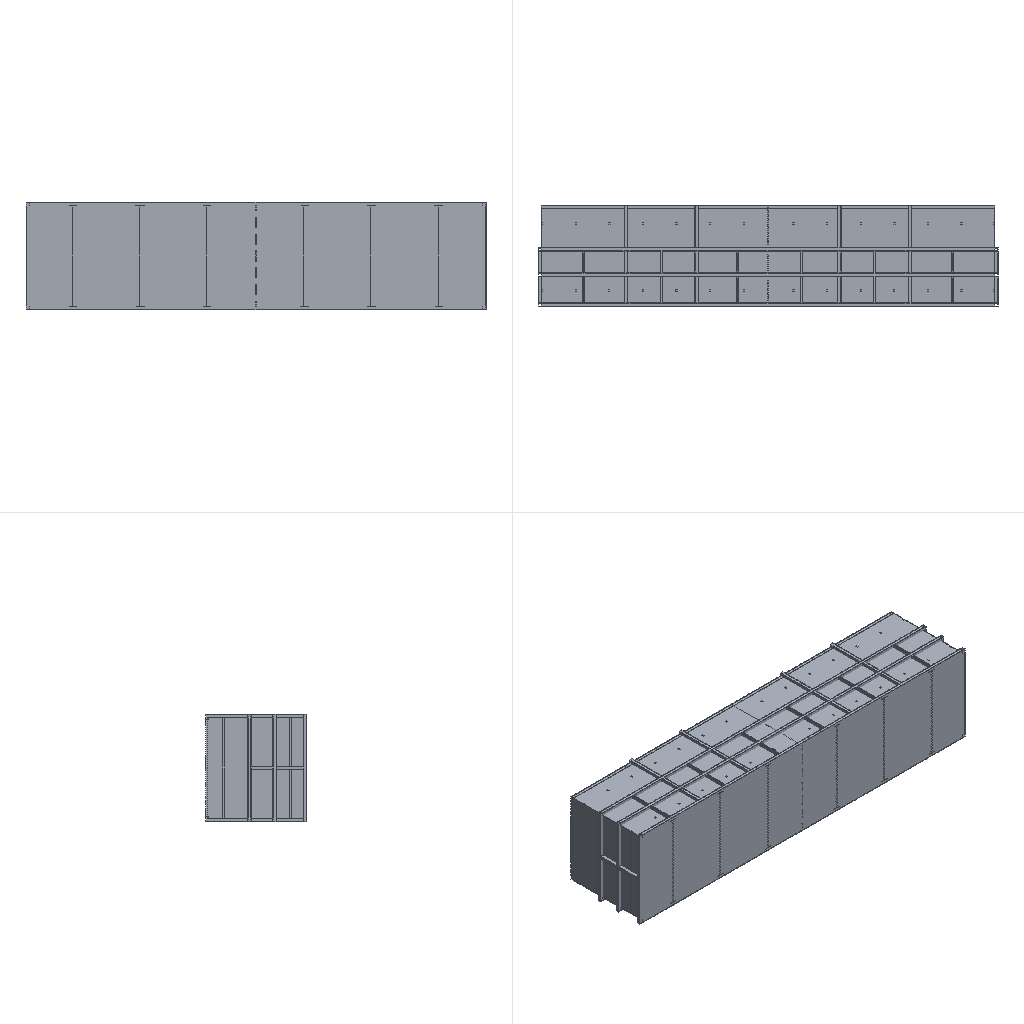Simulation study | ansys workbench
Set-up summary:
category,name,step,type,value,unit,region
solver,ansys_workbench
units,mm-N-s-tonne (MPa),,stated,"/units,MPA"
analysis,LS1,,static
load_step,LS1,LS1,static,nsubst=1; time=1
mesh,nodes,,,1097463
mesh,elements,,,746231
element_type,SOLID187,,,490289
element_type,TARGE170,,,90286
element_type,CONTA174,,,90286
element_type,SURF154,,,57520
element_type,SOLID186,,,17850
material,Structural Steel,,E,200000,tonne s^-2 mm^-1
material,Structural Steel,,nu,0.3
material,Structural Steel,,density,7.85e-09,tonne mm^-3
material,Structural Steel,,conductivity,60.5,tonne mm s^-3 C^-1
material,Structural Steel,,specific_heat,4.34e+08,mm^2 s^-2 C^-1
material,Structural Steel,,cte,1.2e-05,C^-1
material,Structural Steel,,permeability,10000
material,Structural Steel,,resistivity,0.00017,ohm mm
load,Create Hydrostatic Pressure,LS1,pressure,f: 0.0 (MPa),,SURF154 #123
bc,Fixed Supports,model,fixed,[dofs=ALL],,_FIXEDSU
contact,Contact Region,,bonded (always),element=CONTA174
contact,Contact Region 2,,bonded (always),element=CONTA174
contact,Contact Region 3,,bonded (always),element=CONTA174
contact,Contact Region 4,,bonded (always),element=CONTA174
contact,Contact Region 5,,bonded (always),element=CONTA174
contact,Contact Region 6,,bonded (always),element=CONTA174
contact,Contact Region 7,,bonded (always),element=CONTA174
contact,Contact Region 8,,bonded (always),element=CONTA174
contact,Contact Region 9,,bonded (always),element=CONTA174
contact,Contact Region 10,,bonded (always),element=CONTA174
contact,Contact Region 11,,bonded (always),element=CONTA174
contact,Contact Region 12,,bonded (always),element=CONTA174
contact,Contact Region 13,,bonded (always),element=CONTA174
contact,Contact Region 14,,bonded (always),element=CONTA174
contact,Contact Region 15,,bonded (always),element=CONTA174
contact,Contact Region 16,,bonded (always),element=CONTA174
contact,Contact Region 17,,bonded (always),element=CONTA174
contact,Contact Region 18,,bonded (always),element=CONTA174
contact,Contact Region 19,,bonded (always),element=CONTA174
contact,Contact Region 20,,bonded (always),element=CONTA174
contact,Contact Region 21,,bonded (always),element=CONTA174
contact,Contact Region 22,,bonded (always),element=CONTA174
contact,Contact Region 23,,bonded (always),element=CONTA174
contact,Contact Region 24,,bonded (always),element=CONTA174
contact,Contact Region 25,,bonded (always),element=CONTA174
contact,Contact Region 26,,bonded (always),element=CONTA174
contact,Contact Region 27,,bonded (always),element=CONTA174
contact,Contact Region 28,,bonded (always),element=CONTA174
contact,Contact Region 29,,bonded (always),element=CONTA174
contact,Contact Region 30,,bonded (always),element=CONTA174
contact,Contact Region 31,,bonded (always),element=CONTA174
contact,Contact Region 32,,bonded (always),element=CONTA174
contact,Contact Region 33,,bonded (always),element=CONTA174
contact,Contact Region 34,,bonded (always),element=CONTA174
contact,Contact Region 35,,bonded (always),element=CONTA174
contact,Contact Region 36,,bonded (always),element=CONTA174
contact,Contact Region 37,,bonded (always),element=CONTA174
contact,Contact Region 38,,bonded (always),element=CONTA174
contact,Contact Region 39,,bonded (always),element=CONTA174
contact,Contact Region 40,,bonded (always),element=CONTA174
contact,Contact Region 41,,bonded (always),element=CONTA174
contact,Contact Region 42,,bonded (always),element=CONTA174
contact,Contact Region 43,,bonded (always),element=CONTA174
named_set,_FIXEDSU,,node,56341
Ansys APDL input file, long lists of numbers shortened:
/batch
/config,noeldb,1     ! force off writing results to database
*get,_wallstrt,active,,time,wall
! ANSYS input file written by Workbench version 2022 R1
! File used for geometry attach:
/title,wbnew--____ (A5)
! ****** Begin Custom Load Command Snippet ******
/COM, ACT Extensions:
/COM,     LSDYNA, 2021.1
/COM,
! ****** End   Custom Load Command Snippet ******
*DIM,_wb_ProjectScratch_dir,string,248
_wb_ProjectScratch_dir(1) = ''
*DIM,_wb_SolverFiles_dir,string,248
_wb_SolverFiles_dir(1) = ''
*DIM,_wb_userfiles_dir,string,248
_wb_userfiles_dir(1) = ''
/com,--- Data in consistent NMM units. See Solving Units in the help system for more information.
/units,MPA
/nopr
/wb,file,start              !  signify a WB generated input file
/prep7
! Turn off shape checking because checks already performed inside WB mesher.
! See help system for more information.
SHPP,OFF,,NOWARN
/nolist
etcon,set             ! allow ANSYS to choose best KEYOP's for 180x elements, resets any applicable keyopt to MAPDL defaults
/com,*********** Nodes for the whole assembly ***********
nblock,3,,1207209
(1i9,3e20.9e3)
        1    -7.410376924E+02     2.466504369E+03     1.434240000E+03
! (1097462 more lines like these left out)
-1
/wb,elem,start            !  set before creation of elements
/com,*********** Elements for Body 1 "Component2\__-__4" ***********
et,1,187
eblock,19,solid,,318653
(19i9)
        1        1        1        1        0        0        0        0       10        0   189487   459814   468093   474811   466872   567561   624080   567563   567559
! (637305 more lines like these left out)
-1
/com,*********** Elements for Body 2 "Component18\__-__7[6]" ***********
et,2,187
eblock,19,solid,,171636
(19i9)
        2        2        2        2        0        0        0        0       10        0    17851   121406   141417   174356   141306   191452   347128   191456   191450
! (343271 more lines like these left out)
-1
/com,*********** Elements for Body 3 "Component27\C _ 10#(1)[4]" ***********
et,3,186
keyo,3,2,1          ! set full integration on SOLID186
eblock,19,solid,,550
(19i9)
        3        3        3        3        0        0        0        0       20        0     3651    24663    25311    25062    25063    24664    25309    25058    25064
! (1099 more lines like these left out)
-1
/com,*********** Elements for Body 4 "Component28\C _ 10#(1)[3]" ***********
et,4,186
keyo,4,2,1          ! set full integration on SOLID186
eblock,19,solid,,550
(19i9)
        4        4        4        4        0        0        0        0       20        0     5301    36225    36873    36624    36625    36226    36871    36620    36626
! (1099 more lines like these left out)
-1
/com,*********** Elements for Body 5 "Component29\C _ 10#(1)[5]" ***********
et,5,186
keyo,5,2,1          ! set full integration on SOLID186
eblock,19,solid,,550
(19i9)
        5        5        5        5        0        0        0        0       20        0     4201    28517    29165    28916    28917    28518    29163    28912    28918
! (1099 more lines like these left out)
-1
! (31 more sections like these left out)
/wb,elem,end               !  done creating elements
/com,*********** Send User Defined Coordinate System(s) ***********
local,12,0,0.,2800.,0.,-90.,0.,180.
csys,0
toffst,273.15,  ! Temperature offset from absolute zero
/com,*********** Set Reference Temperature ***********
tref,22.
/wb,mat,start              !  starting to send materials
/com,*********** Send Materials ***********
Temperature = 'TEMP' ! Temperature
MP,DENS,1,7.85e-09,	! tonne mm^-3
MP,ALPX,1,1.2e-05,	! C^-1
MP,C,1,434000000,	! mm^2 s^-2 C^-1
MP,KXX,1,60.5,	! tonne mm s^-3 C^-1
MP,RSVX,1,0.00017,	! ohm mm
MP,EX,1,200000,	! tonne s^-2 mm^-1
MP,NUXY,1,0.3,
MP,MURX,1,10000,
Temperature = 'TEMP' ! Temperature
MP,DENS,2,7.85e-09,	! tonne mm^-3
MP,ALPX,2,1.2e-05,	! C^-1
MP,C,2,434000000,	! mm^2 s^-2 C^-1
MP,KXX,2,60.5,	! tonne mm s^-3 C^-1
MP,RSVX,2,0.00017,	! ohm mm
MP,EX,2,200000,	! tonne s^-2 mm^-1
MP,NUXY,2,0.3,
MP,MURX,2,10000,
Temperature = 'TEMP' ! Temperature
MP,DENS,3,7.85e-09,	! tonne mm^-3
MP,ALPX,3,1.2e-05,	! C^-1
MP,C,3,434000000,	! mm^2 s^-2 C^-1
MP,KXX,3,60.5,	! tonne mm s^-3 C^-1
MP,RSVX,3,0.00017,	! ohm mm
MP,EX,3,200000,	! tonne s^-2 mm^-1
MP,NUXY,3,0.3,
MP,MURX,3,10000,
Temperature = 'TEMP' ! Temperature
MP,DENS,4,7.85e-09,	! tonne mm^-3
MP,ALPX,4,1.2e-05,	! C^-1
MP,C,4,434000000,	! mm^2 s^-2 C^-1
MP,KXX,4,60.5,	! tonne mm s^-3 C^-1
MP,RSVX,4,0.00017,	! ohm mm
MP,EX,4,200000,	! tonne s^-2 mm^-1
MP,NUXY,4,0.3,
MP,MURX,4,10000,
Temperature = 'TEMP' ! Temperature
MP,DENS,5,7.85e-09,	! tonne mm^-3
MP,ALPX,5,1.2e-05,	! C^-1
MP,C,5,434000000,	! mm^2 s^-2 C^-1
MP,KXX,5,60.5,	! tonne mm s^-3 C^-1
MP,RSVX,5,0.00017,	! ohm mm
MP,EX,5,200000,	! tonne s^-2 mm^-1
MP,NUXY,5,0.3,
MP,MURX,5,10000,
Temperature = 'TEMP' ! Temperature
MP,DENS,6,7.85e-09,	! tonne mm^-3
MP,ALPX,6,1.2e-05,	! C^-1
MP,C,6,434000000,	! mm^2 s^-2 C^-1
MP,KXX,6,60.5,	! tonne mm s^-3 C^-1
MP,RSVX,6,0.00017,	! ohm mm
MP,EX,6,200000,	! tonne s^-2 mm^-1
MP,NUXY,6,0.3,
MP,MURX,6,10000,
Temperature = 'TEMP' ! Temperature
MP,DENS,7,7.85e-09,	! tonne mm^-3
MP,ALPX,7,1.2e-05,	! C^-1
MP,C,7,434000000,	! mm^2 s^-2 C^-1
MP,KXX,7,60.5,	! tonne mm s^-3 C^-1
MP,RSVX,7,0.00017,	! ohm mm
MP,EX,7,200000,	! tonne s^-2 mm^-1
MP,NUXY,7,0.3,
MP,MURX,7,10000,
Temperature = 'TEMP' ! Temperature
MP,DENS,8,7.85e-09,	! tonne mm^-3
MP,ALPX,8,1.2e-05,	! C^-1
MP,C,8,434000000,	! mm^2 s^-2 C^-1
MP,KXX,8,60.5,	! tonne mm s^-3 C^-1
MP,RSVX,8,0.00017,	! ohm mm
MP,EX,8,200000,	! tonne s^-2 mm^-1
MP,NUXY,8,0.3,
MP,MURX,8,10000,
Temperature = 'TEMP' ! Temperature
MP,DENS,9,7.85e-09,	! tonne mm^-3
MP,ALPX,9,1.2e-05,	! C^-1
MP,C,9,434000000,	! mm^2 s^-2 C^-1
MP,KXX,9,60.5,	! tonne mm s^-3 C^-1
MP,RSVX,9,0.00017,	! ohm mm
MP,EX,9,200000,	! tonne s^-2 mm^-1
! (245 more lines like these left out)
/wb,mat,end                !  done sending materials
!************************* Model Summary ********************
!Component2\__-__4,	结构钢,	matid,	1
!Component18\__-__7[6],	结构钢,	matid,	2
!Component27\C _ 10#(1)[4],	结构钢,	matid,	3
! (35 more lines like these left out)
*get,_xmin,node,,mnloc,x
*get,_ymin,node,,mnloc,y
*get,_zmin,node,,mnloc,z
*get,_xmax,node,,mxloc,x
*get,_ymax,node,,mxloc,y
*get,_zmax,node,,mxloc,z
_ASMDIAG=(_xmax-_xmin)*(_xmax-_xmin)+(_ymax-_ymin)*(_ymax-_ymin)+(_zmax-_zmin)*(_zmax-_zmin)
_ASMDIAG=SQRT(_ASMDIAG)
/wb,contact,start          !  starting to send contact
/com,*********** Create Contact "接触区域" ***********
/com,            Real Constant Set For Above Contact Is 38 & 37
*set,tid,38
*set,cid,37
r,tid
r,cid
et,tid,170
et,cid,174
eblock,10,,,46929
(15i9)
   866282       38       38       38        0   560869   564862   563797   563797  1085489  1095640   563797  1085488
! (46928 more lines like these left out)
-1
eblock,10,,,46929
(15i9)
   913211       37       37       37        0   560869   564862   563797   563797  1085489  1095640   563797  1085488
! (46928 more lines like these left out)
-1
eblock,10,,,26968
(15i9)
   960140       37       38       37        0   123599   143399   173418   173418   209784   355651   173418   209789
! (26967 more lines like these left out)
-1
eblock,10,,,26968
(15i9)
   987108       38       37       38        0   123599   143399   173418   173418   209784   355651   173418   209789
! (26967 more lines like these left out)
-1
keyo,cid,8,2               ! auto create asymmetric contact (from Program Controlled setting)
keyo,cid,10,0              ! adjust contact stiffness each NR iteration (from Program Controlled setting)
keyo,cid,12,5              ! bonded always
keyo,cid,2,2               ! MPC contact.  Valid only for bonded or no separation.  Requires nodal detection
keyo,cid,4,2               ! on nodal point - normal to target surface (from Program Controlled setting)
keyo,cid,9,1               ! ignore initial gaps/penetration
keyo,cid,7,0               ! No Prediction
rmod,tid,3,10.      ! FKN
rmod,tid,5,0.       ! ICONT
rmod,tid,6,-10.     ! PINB
rmod,tid,10,0.      ! CNOF
rmod,tid,12,0.      ! FKT
rmod,tid,36,131     ! WB DSID
rmod,cid,3,10.      ! FKN
rmod,cid,5,0.       ! ICONT
rmod,cid,6,-10.     ! PINB
rmod,cid,10,0.      ! CNOF
rmod,cid,12,0.      ! FKT
rmod,cid,36,131     ! WB DSID
/com,*********** Create Contact "接触区域 2" ***********
/com,            Real Constant Set For Above Contact Is 40 & 39
*set,tid,40
*set,cid,39
r,tid
r,cid
et,tid,170
et,cid,174
eblock,10,,,1067
(15i9)
  1014076       40       40       40        0   560363   561269   565432   565432  1082452  1087494   565432  1082457
! (1066 more lines like these left out)
-1
eblock,10,,,1067
(15i9)
  1015143       39       39       39        0   560363   561269   565432   565432  1082452  1087494   565432  1082457
! (1066 more lines like these left out)
-1
eblock,10,,,322
(15i9)
  1016210       39       40       39        0    24313    25059    24813    24813    25717    27006    24813    25716
! (321 more lines like these left out)
-1
eblock,10,,,322
(15i9)
  1016532       40       39       40        0    24313    25059    24813    24813    25717    27006    24813    25716
! (321 more lines like these left out)
-1
keyo,cid,8,2               ! auto create asymmetric contact (from Program Controlled setting)
keyo,cid,10,0              ! adjust contact stiffness each NR iteration (from Program Controlled setting)
keyo,cid,12,5              ! bonded always
keyo,cid,2,2               ! MPC contact.  Valid only for bonded or no separation.  Requires nodal detection
keyo,cid,4,2               ! on nodal point - normal to target surface (from Program Controlled setting)
keyo,cid,9,1               ! ignore initial gaps/penetration
keyo,cid,7,0               ! No Prediction
rmod,tid,3,10.      ! FKN
rmod,tid,5,0.       ! ICONT
rmod,tid,6,-10.     ! PINB
rmod,tid,10,0.      ! CNOF
rmod,tid,12,0.      ! FKT
rmod,tid,36,134     ! WB DSID
rmod,cid,3,10.      ! FKN
rmod,cid,5,0.       ! ICONT
rmod,cid,6,-10.     ! PINB
rmod,cid,10,0.      ! CNOF
rmod,cid,12,0.      ! FKT
rmod,cid,36,134     ! WB DSID
/com,*********** Create Contact "接触区域 3" ***********
/com,            Real Constant Set For Above Contact Is 42 & 41
*set,tid,42
*set,cid,41
r,tid
r,cid
et,tid,170
et,cid,174
eblock,10,,,1086
(15i9)
  1016854       42       42       42        0   515382   525111   521820   521820   929883   953764   521820   929879
! (1085 more lines like these left out)
-1
eblock,10,,,1086
(15i9)
  1017940       41       41       41        0   515382   525111   521820   521820   929883   953764   521820   929879
! (1085 more lines like these left out)
-1
eblock,10,,,322
(15i9)
  1019026       41       42       41        0    36124    36125    35767    35768    37921    36916    36915    36918
! (321 more lines like these left out)
-1
eblock,10,,,322
(15i9)
  1019348       42       41       42        0    36124    36125    35767    35768    37921    36916    36915    36918
! (321 more lines like these left out)
-1
keyo,cid,8,2               ! auto create asymmetric contact (from Program Controlled setting)
keyo,cid,10,0              ! adjust contact stiffness each NR iteration (from Program Controlled setting)
keyo,cid,12,5              ! bonded always
keyo,cid,2,2               ! MPC contact.  Valid only for bonded or no separation.  Requires nodal detection
keyo,cid,4,2               ! on nodal point - normal to target surface (from Program Controlled setting)
keyo,cid,9,1               ! ignore initial gaps/penetration
keyo,cid,7,0               ! No Prediction
rmod,tid,3,10.      ! FKN
rmod,tid,5,0.       ! ICONT
rmod,tid,6,-10.     ! PINB
rmod,tid,10,0.      ! CNOF
rmod,tid,12,0.      ! FKT
rmod,tid,36,137     ! WB DSID
rmod,cid,3,10.      ! FKN
rmod,cid,5,0.       ! ICONT
rmod,cid,6,-10.     ! PINB
rmod,cid,10,0.      ! CNOF
rmod,cid,12,0.      ! FKT
rmod,cid,36,137     ! WB DSID
/com,*********** Create Contact "接触区域 4" ***********
/com,            Real Constant Set For Above Contact Is 44 & 43
*set,tid,44
*set,cid,43
r,tid
r,cid
et,tid,170
et,cid,174
eblock,10,,,1065
(15i9)
  1019670       44       44       44        0   561874   563090   564356   564356  1090465  1094387   564356  1090467
! (1064 more lines like these left out)
-1
eblock,10,,,1065
(15i9)
  1020735       43       43       43        0   561874   563090   564356   564356  1090465  1094387   564356  1090467
! (1064 more lines like these left out)
-1
eblock,10,,,322
(15i9)
  1021800       43       44       43        0    28167    28913    28667    28667    29571    30860    28667    29570
! (321 more lines like these left out)
-1
eblock,10,,,322
(15i9)
  1022122       44       43       44        0    28167    28913    28667    28667    29571    30860    28667    29570
! (321 more lines like these left out)
-1
keyo,cid,8,2               ! auto create asymmetric contact (from Program Controlled setting)
keyo,cid,10,0              ! adjust contact stiffness each NR iteration (from Program Controlled setting)
keyo,cid,12,5              ! bonded always
keyo,cid,2,2               ! MPC contact.  Valid only for bonded or no separation.  Requires nodal detection
keyo,cid,4,2               ! on nodal point - normal to target surface (from Program Controlled setting)
keyo,cid,9,1               ! ignore initial gaps/penetration
keyo,cid,7,0               ! No Prediction
rmod,tid,3,10.      ! FKN
rmod,tid,5,0.       ! ICONT
rmod,tid,6,-10.     ! PINB
rmod,tid,10,0.      ! CNOF
rmod,tid,12,0.      ! FKT
rmod,tid,36,140     ! WB DSID
rmod,cid,3,10.      ! FKN
rmod,cid,5,0.       ! ICONT
rmod,cid,6,-10.     ! PINB
rmod,cid,10,0.      ! CNOF
rmod,cid,12,0.      ! FKT
rmod,cid,36,140     ! WB DSID
/com,*********** Create Contact "接触区域 5" ***********
/com,            Real Constant Set For Above Contact Is 46 & 45
*set,tid,46
*set,cid,45
r,tid
r,cid
et,tid,170
et,cid,174
eblock,10,,,1126
(15i9)
  1022444       46       46       46        0   515015   520897   522076   522076   927602   951940   522076   927603
! (1125 more lines like these left out)
-1
eblock,10,,,1126
(15i9)
  1023570       45       45       45        0   515015   520897   522076   522076   927602   951940   522076   927603
! (1125 more lines like these left out)
-1
eblock,10,,,322
(15i9)
  1024696       45       46       45        0     7269     7270     6912     6913     9066     8061     8060     8063
! (321 more lines like these left out)
-1
eblock,10,,,322
(15i9)
  1025018       46       45       46        0     7269     7270     6912     6913     9066     8061     8060     8063
! (321 more lines like these left out)
-1
keyo,cid,8,2               ! auto create asymmetric contact (from Program Controlled setting)
keyo,cid,10,0              ! adjust contact stiffness each NR iteration (from Program Controlled setting)
keyo,cid,12,5              ! bonded always
keyo,cid,2,2               ! MPC contact.  Valid only for bonded or no separation.  Requires nodal detection
keyo,cid,4,2               ! on nodal point - normal to target surface (from Program Controlled setting)
keyo,cid,9,1               ! ignore initial gaps/penetration
keyo,cid,7,0               ! No Prediction
rmod,tid,3,10.      ! FKN
rmod,tid,5,0.       ! ICONT
rmod,tid,6,-10.     ! PINB
rmod,tid,10,0.      ! CNOF
rmod,tid,12,0.      ! FKT
rmod,tid,36,143     ! WB DSID
rmod,cid,3,10.      ! FKN
rmod,cid,5,0.       ! ICONT
rmod,cid,6,-10.     ! PINB
rmod,cid,10,0.      ! CNOF
rmod,cid,12,0.      ! FKT
rmod,cid,36,143     ! WB DSID
! (38 more sections like these left out)
/wb,contact,end            !  done creating contacts
/com,*********** Send Named Selection as Element Component ***********
esel,s,type,,1
esel,a,type,,2,36
cm,NONE,elem
esel,all
/golist
/wb,load,start             !  starting to send loads
/com,*********** Fixed Supports ***********
CMBLOCK,_FIXEDSU,NODE,    56341
(8i10)
    463023    463075    463076    463077    463078    463079    463080    463081
! (7042 more lines like these left out)
cmsel,s,_FIXEDSU
d,all,all
nsel,all
/com,*********** Create Hydrostatic Pressure ***********
et,123,154
eblock,10,,,57520
(15i9)
  1046854      123      123      123        0   560869   564862   563797   563797  1085489  1095640   563797  1085488
! (57519 more lines like these left out)
-1
esel,s,type,,123
esel,all
!
! ANSYS Function Representation
!
*DIM,_loadvari270,TABLE,6,9,3,,,,12
!
! Begin of equation: x (MPa)
_loadvari270(0,0,1)= -50, -999
_loadvari270(2,0,1)= 0.0
! (13 more lines like these left out)
! End of equation: x (MPa)
!
! Begin of equation: 9800.*(-x) (MPa)
_loadvari270(0,0,2)= 0, -999
_loadvari270(2,0,2)= 0.0
! (13 more lines like these left out)
! End of equation: 9800.*(-x) (MPa)
!
! Begin of equation: 0.0 (MPa)
_loadvari270(0,0,3)= 50, -999
_loadvari270(2,0,3)= 0.0
! (13 more lines like these left out)
! End of equation: 0.0 (MPa)
!
! ANSYS Function Representation
!
*DIM,_loadvari270r,TABLE,6,12,3,,,,12
!
! Begin of equation: x (MPa)
_loadvari270r(0,0,1)= -50, -999
_loadvari270r(2,0,1)= 0.0
! (16 more lines like these left out)
! End of equation: x (MPa)
!
! Begin of equation: 9800.*(-x)*time/1 (MPa)
_loadvari270r(0,0,2)= 0, -999
_loadvari270r(2,0,2)= 0.0
! (16 more lines like these left out)
! End of equation: 9800.*(-x)*time/1 (MPa)
!
! Begin of equation: 0.0 (MPa)
_loadvari270r(0,0,3)= 50, -999
_loadvari270r(2,0,3)= 0.0
! (16 more lines like these left out)
! End of equation: 0.0 (MPa)
/gst,on,on
fini
*get,_numnode,node,0,count
*get,_numelem,elem,0,count
*get, _MAXELEMNUM, elem, 0, NUM, MAX
*get, _MAXNODENUM, node, 0, NUM, MAX
*get, _MAXELEMTYPE, etyp, 0, NUM, MAX
*get, _MAXREALCONST, real, 0, NUM, MAX
/go
/wb,load,end               !  done creating loads
/com,--- Number of total nodes = %_numnode%
/com,--- Number of contact elements = 238092
/com,--- Number of spring elements = 0
/com,--- Number of bearing elements = 0
/com,--- Number of solid elements = 508139
/com,--- Number of condensed parts = 0
/com,--- Number of total elements = %_numelem%
*get,_wallbsol,active,,time,wall
/com,****************************************************************************
/com,*************************    SOLUTION       ********************************
/com,****************************************************************************
/solu
antype,0                   ! static analysis
neqit,1,force              ! Force 1 eq iteration since only nonlinearity is bonded/no sep contact
pred,off
_thickRatio=0.0278  ! Ratio of thick parts in the model
eqsl,sparse,,,,,1
cntr,print,1               ! print out contact info and also make no initial contact an error
dmpoption,emat,no             ! Don't combine emat file for DANSYS
dmpoption,esav,no             ! Don't combine esav file for DANSYS
nldiag,cont,iter           ! print out contact info each equilibrium iteration
rescontrol,,none                 ! Do not keep any restart files
/com,****************************************************
/com,******************* SOLVE FOR LS 1 OF 1 ****************
esel,s,type,,123
nsle
sf,all,pres,%_loadvari270r%
nsel,all
esel,all
/nopr
/gopr
nsub,1,1,1
time,1.
outres,erase
outres,all,none
outres,nsol,all,
outres,rsol,all
outres,eangl,all
outres,etmp,all
outres,veng,all
outres,strs,all,
outres,epel,all,
outres,eppl,all,
outres,cont,all,
! *********** WB SOLVE COMMAND ***********
! check interactive state
*get,ANSINTER_,active,,int
*if,ANSINTER_,ne,0,then
/eof
*endif
solve
/com *************** Write FE CONNECTORS *********
CEWRITE,file,ce,,INTE
/com,****************************************************
/com,*************** FINISHED SOLVE FOR LS 1 *************
*get,_wallasol,active,,time,wall
/nopr
*get,_numnode,node,0,count
*get,_numelem,elem,0,count
*get, _MAXELEMNUM, elem, 0, NUM, MAX
*get, _MAXNODENUM, node, 0, NUM, MAX,,,INTERNAL
*get, _MAXELEMTYPE, etyp, 0, NUM, MAX
*get, _MAXREALCONST, real, 0, NUM, MAX
/gopr
/post1
xmlo,ENCODING,ISO-8859-1
xmlo,parm
/xml,parm,xml
fini
/gopr
*get,_walldone,active,,time,wall
_preptime=(_wallbsol-_wallstrt)*3600
_solvtime=(_wallasol-_wallbsol)*3600
_posttime=(_walldone-_wallasol)*3600
_totaltim=(_walldone-_wallstrt)*3600
*get,_dlbratio,active,0,solu,dlbr
*get,_combtime,active,0,solu,comb
*get,_ssmode,active,0,solu,ssmm
*get,_ndofs,active,0,solu,ndof
*get,_sol_end_time,active,0,set,time
*if,_sol_end_time,eq,1.,then
/fclean				!clean distributed files
*endif
/com,--- Total number of nodes = %_numnode%
/com,--- Total number of elements = %_numelem%
/com,--- Element load balance ratio = %_dlbratio%
/com,--- Time to combine distributed files = %_combtime%
/com,--- Sparse memory mode = %_ssmode%
/com,--- Number of DOF = %_ndofs%
/wb,file,end               ! done with WB generated input
Results summary:
result,analyses[0].index,,,1
result,analyses[0].system,,,SYS
result,analyses[0].deck,,,deck.dat
result,analyses[0].solve_status,,,completed
result,analyses[0].analysis_type,,,static
result,analyses[0].physics,,,mechanical
result,analyses[0].unit_system,,,"NMM: mm, ton, N, s, mV, mA, degC"
result,analyses[0].n_sets,,,1
result,analyses[0].load_steps[0].set,set=1,,1
result,analyses[0].load_steps[0].time_or_freq,set=1,,1
result,analyses[0].load_steps[0].max_displacement_magnitude,set=1,,5.426
result,analyses[0].load_steps[0].max_von_mises_nodal,set=1,,2.7486e+18
result,analyses[0].load_steps[0].reaction_force_sum_xyz[1],set=1,,0.4299
result,analyses[0].load_steps[0].reaction_force_sum_xyz[2],set=1,,0.0001968
result,analyses[0].load_steps[0].reaction_force_sum_xyz[3],set=1,,-3.828
result,geometry_export[0][0],,,.step
result,geometry_export[0][1],,,ok
result,geometry_export[0][2],,,36